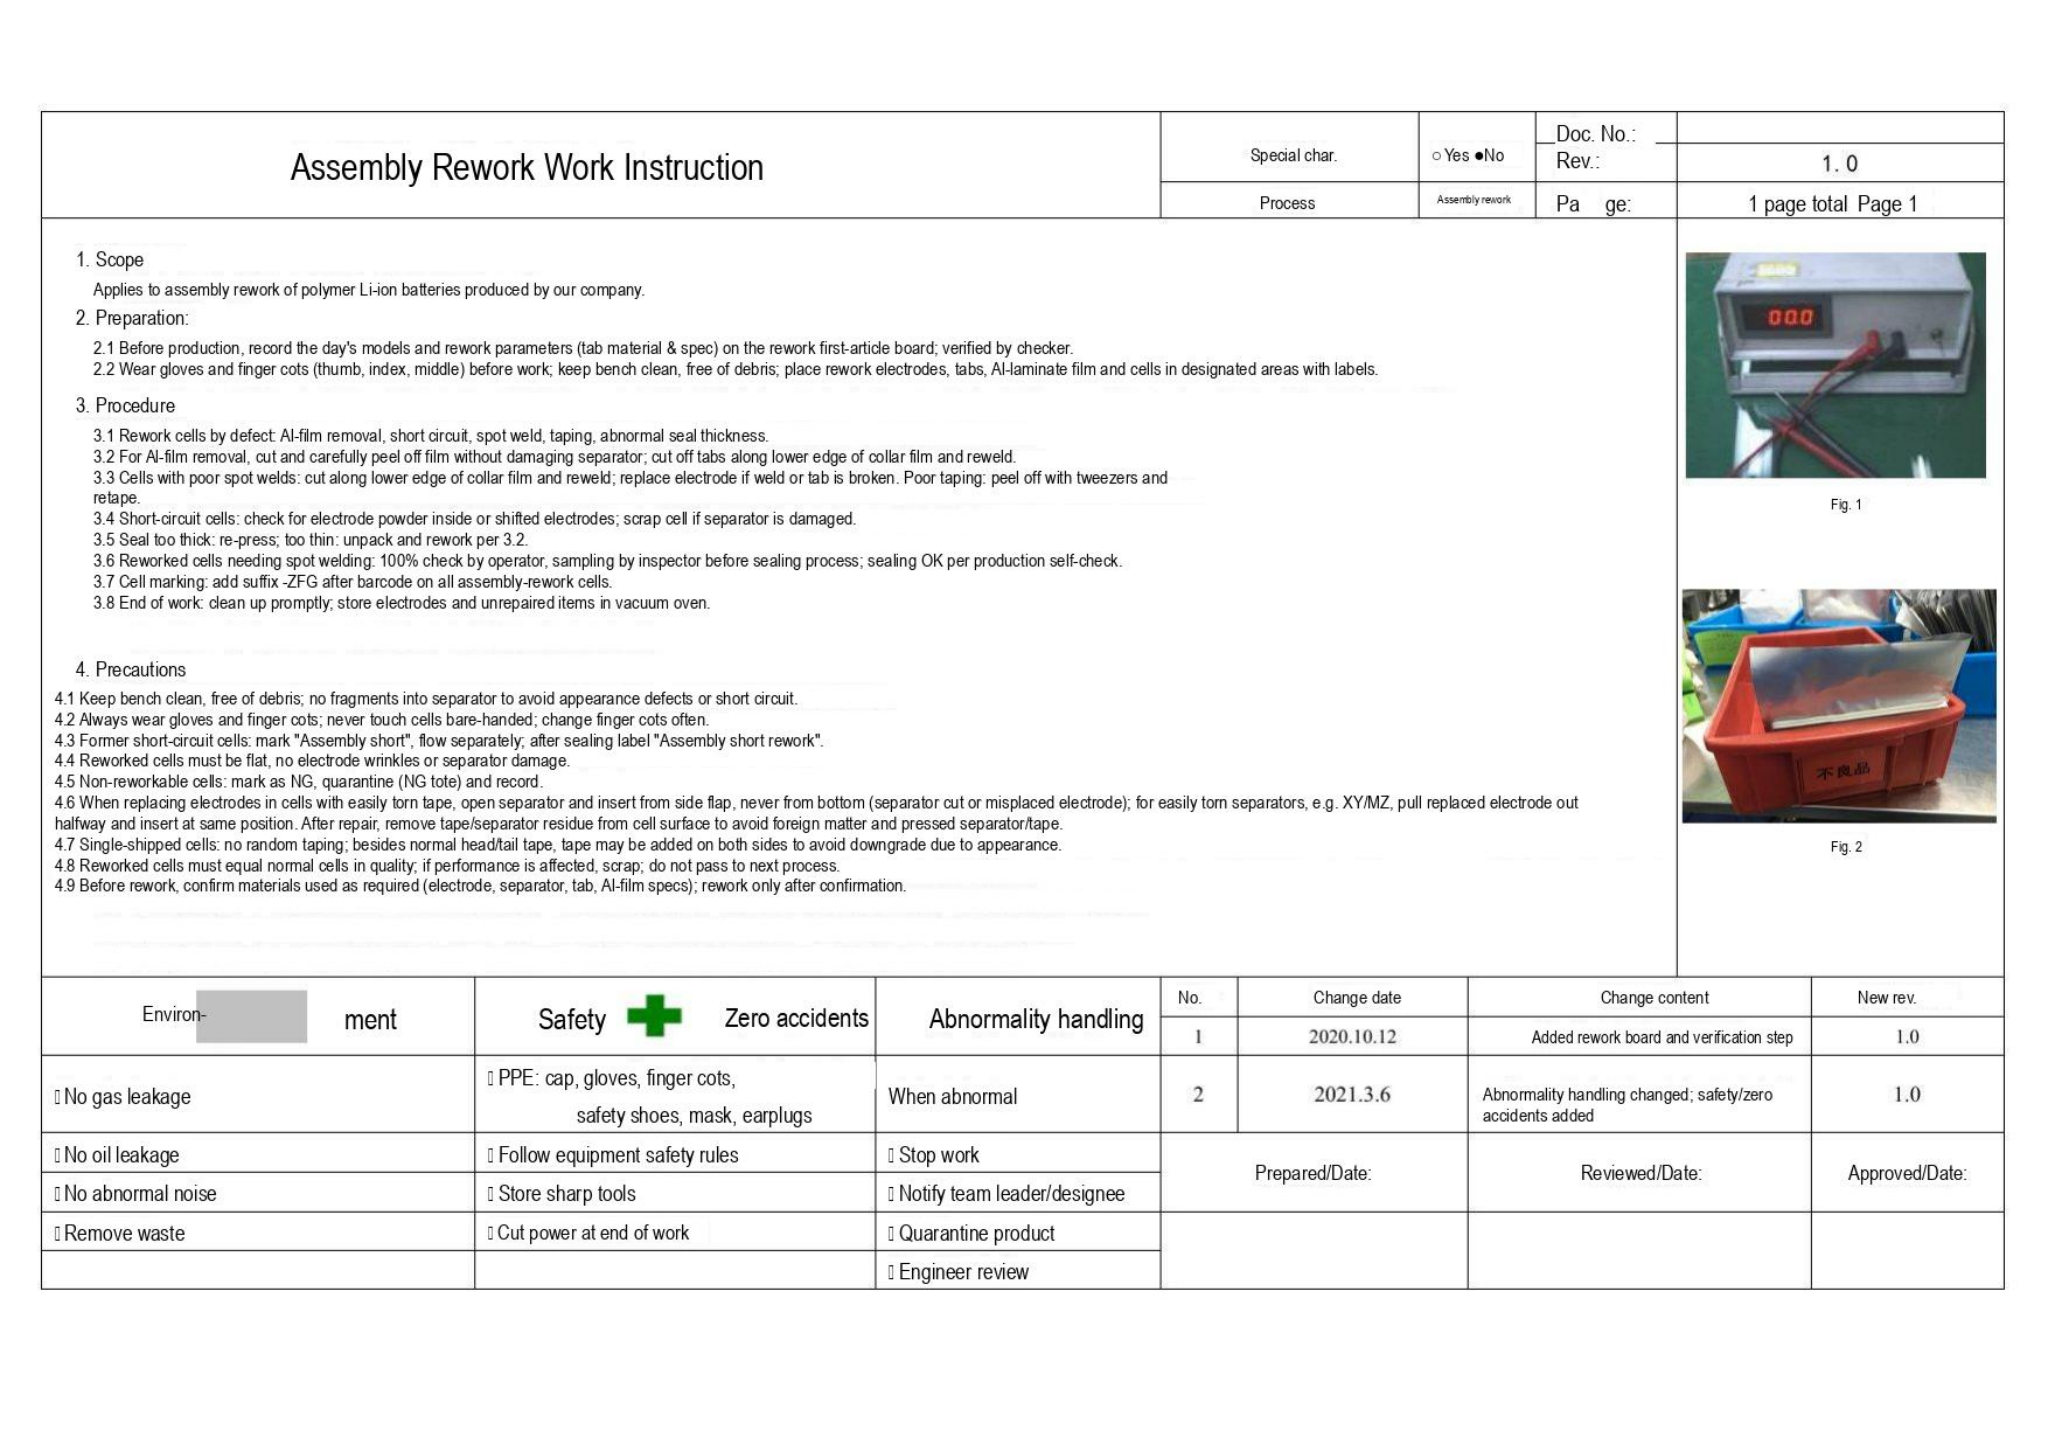# Assembly Rework Work Instruction

| Assembly Rework Work Instruction | Special char. | ○Yes ●No | Doc. No.: | |
|---|---|---|---|---|
| | | | Rev.: | 1. 0 |
| | Process | Assembly rework | Page: | 1 page total Page 1 |

1. Scope

Applies to assembly rework of polymer Li-ion batteries produced by our company.

2. Preparation:

2.1 Before production, record the day's models and rework parameters (tab material & spec) on the rework first-article board; verified by checker.
2.2 Wear gloves and finger cots (thumb, index, middle) before work; keep bench clean, free of debris; place rework electrodes, tabs, Al-laminate film and cells in designated areas with labels.

3. Procedure

3.1 Rework cells by defect: Al-film removal, short circuit, spot weld, taping, abnormal seal thickness.
3.2 For Al-film removal, cut and carefully peel off film without damaging separator; cut off tabs along lower edge of collar film and reweld.
3.3 Cells with poor spot welds: cut along lower edge of collar film and reweld; replace electrode if weld or tab is broken. Poor taping: peel off with tweezers and retape.
3.4 Short-circuit cells: check for electrode powder inside or shifted electrodes; scrap cell if separator is damaged.
3.5 Seal too thick: re-press; too thin: unpack and rework per 3.2.
3.6 Reworked cells needing spot welding: 100% check by operator, sampling by inspector before sealing process; sealing OK per production self-check.
3.7 Cell marking: add suffix -ZFG after barcode on all assembly-rework cells.
3.8 End of work: clean up promptly; store electrodes and unrepaired items in vacuum oven.

4. Precautions

4.1 Keep bench clean, free of debris; no fragments into separator to avoid appearance defects or short circuit.
4.2 Always wear gloves and finger cots; never touch cells bare-handed; change finger cots often.
4.3 Former short-circuit cells: mark "Assembly short", flow separately; after sealing label "Assembly short rework".
4.4 Reworked cells must be flat, no electrode wrinkles or separator damage.
4.5 Non-reworkable cells: mark as NG, quarantine (NG tote) and record.
4.6 When replacing electrodes in cells with easily torn tape, open separator and insert from side flap, never from bottom (separator cut or misplaced electrode); for easily torn separators, e.g. XY/MZ, pull replaced electrode out halfway and insert at same position. After repair, remove tape/separator residue from cell surface to avoid foreign matter and pressed separator/tape.
4.7 Single-shipped cells: no random taping; besides normal head/tail tape, tape may be added on both sides to avoid downgrade due to appearance.
4.8 Reworked cells must equal normal cells in quality; if performance is affected, scrap; do not pass to next process.
4.9 Before rework, confirm materials used as required (electrode, separator, tab, Al-film specs); rework only after confirmation.

Fig. 1

不良品

Fig. 2

| Environ- ment | Safety Zero accidents | Abnormality handling |
|---|---|---|
| ▯No gas leakage | ▯PPE: cap, gloves, finger cots, safety shoes, mask, earplugs | When abnormal |
| ▯No oil leakage | ▯Follow equipment safety rules | ▯Stop work |
| ▯No abnormal noise | ▯Store sharp tools | ▯Notify team leader/designee |
| ▯Remove waste | ▯Cut power at end of work | ▯Quarantine product |
| | | ▯Engineer review |

| No. | Change date | Change content | New rev. |
|---|---|---|---|
| 1 | 2020.10.12 | Added rework board and verification step | 1.0 |
| 2 | 2021.3.6 | Abnormality handling changed; safety/zero accidents added | 1.0 |

| Prepared/Date: | Reviewed/Date: | Approved/Date: |
|---|---|---|
| | | |